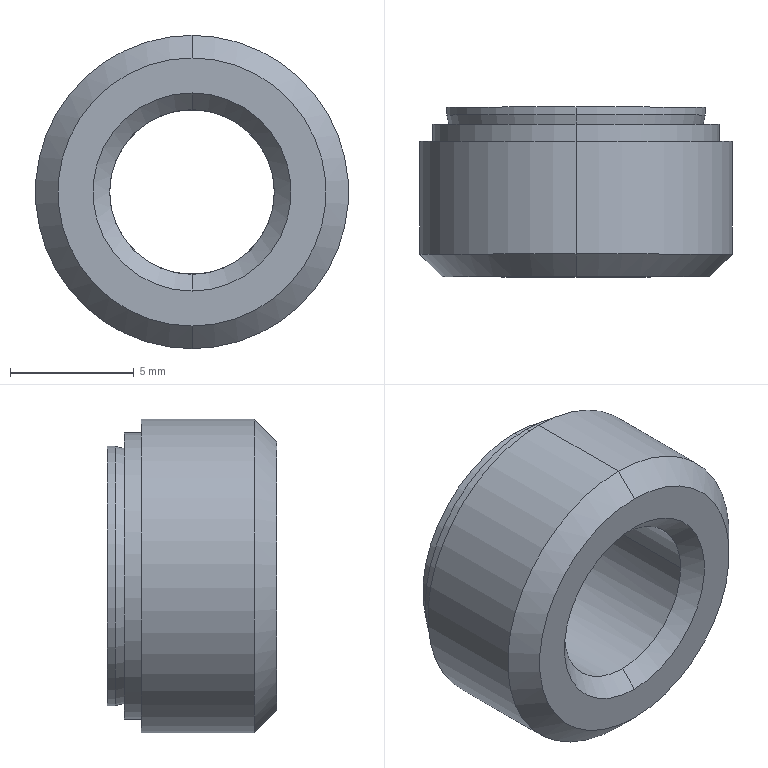Part | NX | features solid 2 | 1 solid | 20 faces | box 12.65 x 6.85 x 12.65 mm | volume 555.144 mm3 | cone 8 | cylinder 8 | plane 4 | commonest cylinder face diameters 6.647 x2 10.47 x2 11.56 x2 12.65 x2
STEP:
#1=CARTESIAN_POINT('',(107.,-8.66,-1026.113));
#2=VERTEX_POINT('',#1);
#3=CARTESIAN_POINT('',(107.,-8.66,-1015.287));
#4=VERTEX_POINT('',#3);
#5=CARTESIAN_POINT('',(107.,-8.66,-1020.7));
#6=DIRECTION('',(0.,1.,0.));
#7=DIRECTION('',(0.,0.,-1.));
#8=AXIS2_PLACEMENT_3D('',#5,#6,#7);
#9=CIRCLE('',#8,5.413);
#10=EDGE_CURVE('',#2,#4,#9,.T.);
#11=ORIENTED_EDGE('',*,*,#10,.T.);
#12=CARTESIAN_POINT('',(107.,-7.748,-1014.375));
#13=VERTEX_POINT('',#12);
#14=CARTESIAN_POINT('',(107.,-7.748,-1014.375));
#15=DIRECTION('',(0.,-0.7071,-0.7071));
#16=VECTOR('',#15,1000.);
#17=LINE('',#14,#16);
#18=EDGE_CURVE('',#4,#13,#17,.F.);
#19=ORIENTED_EDGE('',*,*,#18,.T.);
#20=CARTESIAN_POINT('',(107.,-7.748,-1027.025));
#21=VERTEX_POINT('',#20);
#22=CARTESIAN_POINT('',(107.,-7.748,-1020.7));
#23=DIRECTION('',(0.,1.,0.));
#24=DIRECTION('',(0.,0.,-1.));
#25=AXIS2_PLACEMENT_3D('',#22,#23,#24);
#26=CIRCLE('',#25,6.325);
#27=EDGE_CURVE('',#21,#13,#26,.T.);
#28=ORIENTED_EDGE('',*,*,#27,.F.);
#29=CARTESIAN_POINT('',(107.,-7.748,-1027.025));
#30=DIRECTION('',(0.,-0.7071,0.7071));
#31=VECTOR('',#30,1000.);
#32=LINE('',#29,#31);
#33=EDGE_CURVE('',#21,#2,#32,.T.);
#34=ORIENTED_EDGE('',*,*,#33,.T.);
#35=EDGE_LOOP('',(#11,#19,#28,#34));
#36=FACE_BOUND('',#35,.T.);
#37=CARTESIAN_POINT('',(107.,-8.204,-1020.7));
#38=DIRECTION('',(0.,1.,0.));
#39=DIRECTION('',(0.,0.,-1.));
#40=AXIS2_PLACEMENT_3D('',#37,#38,#39);
#41=CONICAL_SURFACE('',#40,5.869,0.7854);
#42=ADVANCED_FACE('',(#36),#41,.T.);
#43=ORIENTED_EDGE('',*,*,#33,.F.);
#44=CARTESIAN_POINT('',(107.,-7.748,-1020.7));
#45=DIRECTION('',(0.,1.,0.));
#46=DIRECTION('',(0.,0.,1.));
#47=AXIS2_PLACEMENT_3D('',#44,#45,#46);
#48=CIRCLE('',#47,6.325);
#49=EDGE_CURVE('',#13,#21,#48,.T.);
#50=ORIENTED_EDGE('',*,*,#49,.F.);
#51=ORIENTED_EDGE('',*,*,#18,.F.);
#52=CARTESIAN_POINT('',(107.,-8.66,-1020.7));
#53=DIRECTION('',(0.,1.,0.));
#54=DIRECTION('',(0.,0.,1.));
#55=AXIS2_PLACEMENT_3D('',#52,#53,#54);
#56=CIRCLE('',#55,5.413);
#57=EDGE_CURVE('',#4,#2,#56,.T.);
#58=ORIENTED_EDGE('',*,*,#57,.T.);
#59=EDGE_LOOP('',(#43,#50,#51,#58));
#60=FACE_BOUND('',#59,.T.);
#61=CARTESIAN_POINT('',(107.,-8.204,-1020.7));
#62=DIRECTION('',(0.,1.,0.));
#63=DIRECTION('',(0.,0.,-1.));
#64=AXIS2_PLACEMENT_3D('',#61,#62,#63);
#65=CONICAL_SURFACE('',#64,5.869,0.7854);
#66=ADVANCED_FACE('',(#60),#65,.T.);
#67=ORIENTED_EDGE('',*,*,#10,.F.);
#68=ORIENTED_EDGE('',*,*,#57,.F.);
#69=EDGE_LOOP('',(#67,#68));
#70=FACE_BOUND('',#69,.T.);
#71=CARTESIAN_POINT('',(107.,-8.66,-1024.7));
#72=VERTEX_POINT('',#71);
#73=CARTESIAN_POINT('',(107.,-8.66,-1016.7));
#74=VERTEX_POINT('',#73);
#75=CARTESIAN_POINT('',(107.,-8.66,-1020.7));
#76=DIRECTION('',(0.,-1.,0.));
#77=DIRECTION('',(0.,0.,-1.));
#78=AXIS2_PLACEMENT_3D('',#75,#76,#77);
#79=CIRCLE('',#78,4.);
#80=EDGE_CURVE('',#72,#74,#79,.T.);
#81=ORIENTED_EDGE('',*,*,#80,.F.);
#82=CARTESIAN_POINT('',(107.,-8.66,-1020.7));
#83=DIRECTION('',(0.,-1.,0.));
#84=DIRECTION('',(0.,0.,1.));
#85=AXIS2_PLACEMENT_3D('',#82,#83,#84);
#86=CIRCLE('',#85,4.);
#87=EDGE_CURVE('',#74,#72,#86,.T.);
#88=ORIENTED_EDGE('',*,*,#87,.F.);
#89=EDGE_LOOP('',(#81,#88));
#90=FACE_BOUND('',#89,.T.);
#91=CARTESIAN_POINT('',(107.,-8.66,-1017.993));
#92=DIRECTION('',(0.,-1.,0.));
#93=DIRECTION('',(-1.,0.,0.));
#94=AXIS2_PLACEMENT_3D('',#91,#92,#93);
#95=PLANE('',#94);
#96=ADVANCED_FACE('',(#70,#90),#95,.T.);
#97=CARTESIAN_POINT('',(107.,-7.984,-1017.377));
#98=VERTEX_POINT('',#97);
#99=CARTESIAN_POINT('',(107.,-8.66,-1016.7));
#100=DIRECTION('',(0.,0.7071,-0.7071));
#101=VECTOR('',#100,1000.);
#102=LINE('',#99,#101);
#103=EDGE_CURVE('',#74,#98,#102,.T.);
#104=ORIENTED_EDGE('',*,*,#103,.F.);
#105=ORIENTED_EDGE('',*,*,#87,.T.);
#106=CARTESIAN_POINT('',(107.,-7.984,-1024.023));
#107=VERTEX_POINT('',#106);
#108=CARTESIAN_POINT('',(107.,-8.66,-1024.7));
#109=DIRECTION('',(0.,0.7071,0.7071));
#110=VECTOR('',#109,1000.);
#111=LINE('',#108,#110);
#112=EDGE_CURVE('',#107,#72,#111,.F.);
#113=ORIENTED_EDGE('',*,*,#112,.F.);
#114=CARTESIAN_POINT('',(103.677,-7.984,-1020.7));
#115=VERTEX_POINT('',#114);
#116=CARTESIAN_POINT('',(107.,-7.984,-1020.7));
#117=DIRECTION('',(0.,-1.,0.));
#118=DIRECTION('',(-1.,0.,0.));
#119=AXIS2_PLACEMENT_3D('',#116,#117,#118);
#120=CIRCLE('',#119,3.323);
#121=EDGE_CURVE('',#115,#107,#120,.T.);
#122=ORIENTED_EDGE('',*,*,#121,.F.);
#123=CARTESIAN_POINT('',(107.,-7.984,-1020.7));
#124=DIRECTION('',(0.,-1.,0.));
#125=DIRECTION('',(0.,0.,1.));
#126=AXIS2_PLACEMENT_3D('',#123,#124,#125);
#127=CIRCLE('',#126,3.323);
#128=EDGE_CURVE('',#98,#115,#127,.T.);
#129=ORIENTED_EDGE('',*,*,#128,.F.);
#130=EDGE_LOOP('',(#104,#105,#113,#122,#129));
#131=FACE_BOUND('',#130,.T.);
#132=CARTESIAN_POINT('',(107.,-8.322,-1020.7));
#133=DIRECTION('',(0.,-1.,0.));
#134=DIRECTION('',(0.,0.,1.));
#135=AXIS2_PLACEMENT_3D('',#132,#133,#134);
#136=CONICAL_SURFACE('',#135,3.662,0.7854);
#137=ADVANCED_FACE('',(#131),#136,.F.);
#138=CARTESIAN_POINT('',(110.323,-7.984,-1020.7));
#139=VERTEX_POINT('',#138);
#140=CARTESIAN_POINT('',(107.,-7.984,-1020.7));
#141=DIRECTION('',(0.,-1.,0.));
#142=DIRECTION('',(1.,0.,0.));
#143=AXIS2_PLACEMENT_3D('',#140,#141,#142);
#144=CIRCLE('',#143,3.323);
#145=EDGE_CURVE('',#139,#98,#144,.T.);
#146=ORIENTED_EDGE('',*,*,#145,.T.);
#147=ORIENTED_EDGE('',*,*,#128,.T.);
#148=CARTESIAN_POINT('',(103.676,-2.487,-1020.7));
#149=VERTEX_POINT('',#148);
#150=CARTESIAN_POINT('',(103.676,-2.487,-1020.7));
#151=DIRECTION('',(0.,-1.,0.));
#152=VECTOR('',#151,1000.);
#153=LINE('',#150,#152);
#154=EDGE_CURVE('',#149,#115,#153,.T.);
#155=ORIENTED_EDGE('',*,*,#154,.F.);
#156=CARTESIAN_POINT('',(110.324,-2.487,-1020.7));
#157=VERTEX_POINT('',#156);
#158=CARTESIAN_POINT('',(107.,-2.487,-1020.7));
#159=DIRECTION('',(0.,1.,0.));
#160=DIRECTION('',(-1.,0.,0.));
#161=AXIS2_PLACEMENT_3D('',#158,#159,#160);
#162=CIRCLE('',#161,3.324);
#163=EDGE_CURVE('',#149,#157,#162,.T.);
#164=ORIENTED_EDGE('',*,*,#163,.T.);
#165=CARTESIAN_POINT('',(110.324,-2.487,-1020.7));
#166=DIRECTION('',(0.,-1.,0.));
#167=VECTOR('',#166,1000.);
#168=LINE('',#165,#167);
#169=EDGE_CURVE('',#139,#157,#168,.F.);
#170=ORIENTED_EDGE('',*,*,#169,.F.);
#171=EDGE_LOOP('',(#146,#147,#155,#164,#170));
#172=FACE_BOUND('',#171,.T.);
#173=CARTESIAN_POINT('',(107.,-7.984,-1020.7));
#174=DIRECTION('',(0.,1.,0.));
#175=DIRECTION('',(1.,0.,0.));
#176=AXIS2_PLACEMENT_3D('',#173,#174,#175);
#177=CYLINDRICAL_SURFACE('',#176,3.324);
#178=ADVANCED_FACE('',(#172),#177,.F.);
#179=ORIENTED_EDGE('',*,*,#169,.T.);
#180=CARTESIAN_POINT('',(107.,-2.487,-1020.7));
#181=DIRECTION('',(0.,1.,0.));
#182=DIRECTION('',(1.,0.,0.));
#183=AXIS2_PLACEMENT_3D('',#180,#181,#182);
#184=CIRCLE('',#183,3.324);
#185=EDGE_CURVE('',#157,#149,#184,.T.);
#186=ORIENTED_EDGE('',*,*,#185,.T.);
#187=ORIENTED_EDGE('',*,*,#154,.T.);
#188=ORIENTED_EDGE('',*,*,#121,.T.);
#189=CARTESIAN_POINT('',(107.,-7.984,-1020.7));
#190=DIRECTION('',(0.,-1.,0.));
#191=DIRECTION('',(0.,0.,-1.));
#192=AXIS2_PLACEMENT_3D('',#189,#190,#191);
#193=CIRCLE('',#192,3.323);
#194=EDGE_CURVE('',#107,#139,#193,.T.);
#195=ORIENTED_EDGE('',*,*,#194,.T.);
#196=EDGE_LOOP('',(#179,#186,#187,#188,#195));
#197=FACE_BOUND('',#196,.T.);
#198=CARTESIAN_POINT('',(107.,-7.984,-1020.7));
#199=DIRECTION('',(0.,1.,0.));
#200=DIRECTION('',(1.,0.,0.));
#201=AXIS2_PLACEMENT_3D('',#198,#199,#200);
#202=CYLINDRICAL_SURFACE('',#201,3.324);
#203=ADVANCED_FACE('',(#197),#202,.F.);
#204=ORIENTED_EDGE('',*,*,#145,.F.);
#205=ORIENTED_EDGE('',*,*,#194,.F.);
#206=ORIENTED_EDGE('',*,*,#112,.T.);
#207=ORIENTED_EDGE('',*,*,#80,.T.);
#208=ORIENTED_EDGE('',*,*,#103,.T.);
#209=EDGE_LOOP('',(#204,#205,#206,#207,#208));
#210=FACE_BOUND('',#209,.T.);
#211=CARTESIAN_POINT('',(107.,-8.322,-1020.7));
#212=DIRECTION('',(0.,-1.,0.));
#213=DIRECTION('',(0.,0.,1.));
#214=AXIS2_PLACEMENT_3D('',#211,#212,#213);
#215=CONICAL_SURFACE('',#214,3.662,0.7854);
#216=ADVANCED_FACE('',(#210),#215,.F.);
#217=CARTESIAN_POINT('',(111.,-1.81,-1020.7));
#218=VERTEX_POINT('',#217);
#219=CARTESIAN_POINT('',(111.,-1.81,-1020.7));
#220=DIRECTION('',(-0.7071,-0.7071,0.));
#221=VECTOR('',#220,1000.);
#222=LINE('',#219,#221);
#223=EDGE_CURVE('',#157,#218,#222,.F.);
#224=ORIENTED_EDGE('',*,*,#223,.T.);
#225=CARTESIAN_POINT('',(103.,-1.81,-1020.7));
#226=VERTEX_POINT('',#225);
#227=CARTESIAN_POINT('',(107.,-1.81,-1020.7));
#228=DIRECTION('',(0.,1.,0.));
#229=DIRECTION('',(1.,0.,0.));
#230=AXIS2_PLACEMENT_3D('',#227,#228,#229);
#231=CIRCLE('',#230,4.);
#232=EDGE_CURVE('',#218,#226,#231,.T.);
#233=ORIENTED_EDGE('',*,*,#232,.T.);
#234=CARTESIAN_POINT('',(103.,-1.81,-1020.7));
#235=DIRECTION('',(0.7071,-0.7071,0.));
#236=VECTOR('',#235,1000.);
#237=LINE('',#234,#236);
#238=EDGE_CURVE('',#226,#149,#237,.T.);
#239=ORIENTED_EDGE('',*,*,#238,.T.);
#240=ORIENTED_EDGE('',*,*,#185,.F.);
#241=EDGE_LOOP('',(#224,#233,#239,#240));
#242=FACE_BOUND('',#241,.T.);
#243=CARTESIAN_POINT('',(107.,-2.148,-1020.7));
#244=DIRECTION('',(0.,1.,0.));
#245=DIRECTION('',(1.,0.,0.));
#246=AXIS2_PLACEMENT_3D('',#243,#244,#245);
#247=CONICAL_SURFACE('',#246,3.662,0.7854);
#248=ADVANCED_FACE('',(#242),#247,.F.);
#249=ORIENTED_EDGE('',*,*,#163,.F.);
#250=ORIENTED_EDGE('',*,*,#238,.F.);
#251=CARTESIAN_POINT('',(107.,-1.81,-1020.7));
#252=DIRECTION('',(0.,1.,0.));
#253=DIRECTION('',(-1.,0.,0.));
#254=AXIS2_PLACEMENT_3D('',#251,#252,#253);
#255=CIRCLE('',#254,4.);
#256=EDGE_CURVE('',#226,#218,#255,.T.);
#257=ORIENTED_EDGE('',*,*,#256,.T.);
#258=ORIENTED_EDGE('',*,*,#223,.F.);
#259=EDGE_LOOP('',(#249,#250,#257,#258));
#260=FACE_BOUND('',#259,.T.);
#261=CARTESIAN_POINT('',(107.,-2.148,-1020.7));
#262=DIRECTION('',(0.,1.,0.));
#263=DIRECTION('',(1.,0.,0.));
#264=AXIS2_PLACEMENT_3D('',#261,#262,#263);
#265=CONICAL_SURFACE('',#264,3.662,0.7854);
#266=ADVANCED_FACE('',(#260),#265,.F.);
#267=CARTESIAN_POINT('',(107.,-1.81,-1015.465));
#268=VERTEX_POINT('',#267);
#269=CARTESIAN_POINT('',(107.,-1.81,-1025.935));
#270=VERTEX_POINT('',#269);
#271=CARTESIAN_POINT('',(107.,-1.81,-1020.7));
#272=DIRECTION('',(0.,-1.,0.));
#273=DIRECTION('',(0.,0.,1.));
#274=AXIS2_PLACEMENT_3D('',#271,#272,#273);
#275=CIRCLE('',#274,5.235);
#276=EDGE_CURVE('',#268,#270,#275,.T.);
#277=ORIENTED_EDGE('',*,*,#276,.F.);
#278=CARTESIAN_POINT('',(107.,-1.81,-1020.7));
#279=DIRECTION('',(0.,-1.,0.));
#280=DIRECTION('',(0.,0.,-1.));
#281=AXIS2_PLACEMENT_3D('',#278,#279,#280);
#282=CIRCLE('',#281,5.235);
#283=EDGE_CURVE('',#270,#268,#282,.T.);
#284=ORIENTED_EDGE('',*,*,#283,.F.);
#285=EDGE_LOOP('',(#277,#284));
#286=FACE_BOUND('',#285,.T.);
#287=ORIENTED_EDGE('',*,*,#232,.F.);
#288=ORIENTED_EDGE('',*,*,#256,.F.);
#289=EDGE_LOOP('',(#287,#288));
#290=FACE_BOUND('',#289,.T.);
#291=CARTESIAN_POINT('',(107.,-1.81,-1018.082));
#292=DIRECTION('',(0.,1.,0.));
#293=DIRECTION('',(0.,0.,-1.));
#294=AXIS2_PLACEMENT_3D('',#291,#292,#293);
#295=PLANE('',#294);
#296=ADVANCED_FACE('',(#286,#290),#295,.T.);
#297=CARTESIAN_POINT('',(107.,-2.128,-1015.465));
#298=VERTEX_POINT('',#297);
#299=CARTESIAN_POINT('',(107.,-2.128,-1015.465));
#300=DIRECTION('',(0.,1.,0.));
#301=VECTOR('',#300,1000.);
#302=LINE('',#299,#301);
#303=EDGE_CURVE('',#268,#298,#302,.F.);
#304=ORIENTED_EDGE('',*,*,#303,.T.);
#305=CARTESIAN_POINT('',(107.,-2.128,-1025.935));
#306=VERTEX_POINT('',#305);
#307=CARTESIAN_POINT('',(107.,-2.128,-1020.7));
#308=DIRECTION('',(0.,1.,0.));
#309=DIRECTION('',(0.,0.,1.));
#310=AXIS2_PLACEMENT_3D('',#307,#308,#309);
#311=CIRCLE('',#310,5.235);
#312=EDGE_CURVE('',#298,#306,#311,.T.);
#313=ORIENTED_EDGE('',*,*,#312,.T.);
#314=CARTESIAN_POINT('',(107.,-2.128,-1025.935));
#315=DIRECTION('',(0.,1.,0.));
#316=VECTOR('',#315,1000.);
#317=LINE('',#314,#316);
#318=EDGE_CURVE('',#306,#270,#317,.T.);
#319=ORIENTED_EDGE('',*,*,#318,.T.);
#320=ORIENTED_EDGE('',*,*,#283,.T.);
#321=EDGE_LOOP('',(#304,#313,#319,#320));
#322=FACE_BOUND('',#321,.T.);
#323=CARTESIAN_POINT('',(107.,-1.969,-1020.7));
#324=DIRECTION('',(0.,-1.,0.));
#325=DIRECTION('',(0.,0.,1.));
#326=AXIS2_PLACEMENT_3D('',#323,#324,#325);
#327=CYLINDRICAL_SURFACE('',#326,5.235);
#328=ADVANCED_FACE('',(#322),#327,.T.);
#329=ORIENTED_EDGE('',*,*,#276,.T.);
#330=ORIENTED_EDGE('',*,*,#318,.F.);
#331=CARTESIAN_POINT('',(107.,-2.128,-1020.7));
#332=DIRECTION('',(0.,1.,0.));
#333=DIRECTION('',(0.,0.,-1.));
#334=AXIS2_PLACEMENT_3D('',#331,#332,#333);
#335=CIRCLE('',#334,5.235);
#336=EDGE_CURVE('',#306,#298,#335,.T.);
#337=ORIENTED_EDGE('',*,*,#336,.T.);
#338=ORIENTED_EDGE('',*,*,#303,.F.);
#339=EDGE_LOOP('',(#329,#330,#337,#338));
#340=FACE_BOUND('',#339,.T.);
#341=CARTESIAN_POINT('',(107.,-1.969,-1020.7));
#342=DIRECTION('',(0.,-1.,0.));
#343=DIRECTION('',(0.,0.,1.));
#344=AXIS2_PLACEMENT_3D('',#341,#342,#343);
#345=CYLINDRICAL_SURFACE('',#344,5.235);
#346=ADVANCED_FACE('',(#340),#345,.T.);
#347=CARTESIAN_POINT('',(107.,-2.5,-1025.848));
#348=VERTEX_POINT('',#347);
#349=CARTESIAN_POINT('',(107.,-2.5,-1015.552));
#350=VERTEX_POINT('',#349);
#351=CARTESIAN_POINT('',(107.,-2.5,-1020.7));
#352=DIRECTION('',(0.,1.,0.));
#353=DIRECTION('',(0.,0.,-1.));
#354=AXIS2_PLACEMENT_3D('',#351,#352,#353);
#355=CIRCLE('',#354,5.148);
#356=EDGE_CURVE('',#348,#350,#355,.T.);
#357=ORIENTED_EDGE('',*,*,#356,.T.);
#358=CARTESIAN_POINT('',(107.,-2.128,-1015.465));
#359=DIRECTION('',(0.,-0.9735,-0.2286));
#360=VECTOR('',#359,1000.);
#361=LINE('',#358,#360);
#362=EDGE_CURVE('',#350,#298,#361,.F.);
#363=ORIENTED_EDGE('',*,*,#362,.T.);
#364=ORIENTED_EDGE('',*,*,#336,.F.);
#365=CARTESIAN_POINT('',(107.,-2.128,-1025.935));
#366=DIRECTION('',(0.,-0.9735,0.2286));
#367=VECTOR('',#366,1000.);
#368=LINE('',#365,#367);
#369=EDGE_CURVE('',#306,#348,#368,.T.);
#370=ORIENTED_EDGE('',*,*,#369,.T.);
#371=EDGE_LOOP('',(#357,#363,#364,#370));
#372=FACE_BOUND('',#371,.T.);
#373=CARTESIAN_POINT('',(107.,-2.314,-1020.7));
#374=DIRECTION('',(0.,1.,0.));
#375=DIRECTION('',(0.,0.,-1.));
#376=AXIS2_PLACEMENT_3D('',#373,#374,#375);
#377=CONICAL_SURFACE('',#376,5.191,0.2307);
#378=ADVANCED_FACE('',(#372),#377,.T.);
#379=ORIENTED_EDGE('',*,*,#369,.F.);
#380=ORIENTED_EDGE('',*,*,#312,.F.);
#381=ORIENTED_EDGE('',*,*,#362,.F.);
#382=CARTESIAN_POINT('',(107.,-2.5,-1020.7));
#383=DIRECTION('',(0.,1.,0.));
#384=DIRECTION('',(0.,0.,1.));
#385=AXIS2_PLACEMENT_3D('',#382,#383,#384);
#386=CIRCLE('',#385,5.148);
#387=EDGE_CURVE('',#350,#348,#386,.T.);
#388=ORIENTED_EDGE('',*,*,#387,.T.);
#389=EDGE_LOOP('',(#379,#380,#381,#388));
#390=FACE_BOUND('',#389,.T.);
#391=CARTESIAN_POINT('',(107.,-2.314,-1020.7));
#392=DIRECTION('',(0.,1.,0.));
#393=DIRECTION('',(0.,0.,-1.));
#394=AXIS2_PLACEMENT_3D('',#391,#392,#393);
#395=CONICAL_SURFACE('',#394,5.191,0.2307);
#396=ADVANCED_FACE('',(#390),#395,.T.);
#397=CARTESIAN_POINT('',(107.,-2.5,-1026.48));
#398=VERTEX_POINT('',#397);
#399=CARTESIAN_POINT('',(107.,-2.5,-1014.92));
#400=VERTEX_POINT('',#399);
#401=CARTESIAN_POINT('',(107.,-2.5,-1020.7));
#402=DIRECTION('',(0.,-1.,0.));
#403=DIRECTION('',(0.,0.,-1.));
#404=AXIS2_PLACEMENT_3D('',#401,#402,#403);
#405=CIRCLE('',#404,5.78);
#406=EDGE_CURVE('',#398,#400,#405,.T.);
#407=ORIENTED_EDGE('',*,*,#406,.F.);
#408=CARTESIAN_POINT('',(107.,-2.5,-1020.7));
#409=DIRECTION('',(0.,-1.,0.));
#410=DIRECTION('',(0.,0.,1.));
#411=AXIS2_PLACEMENT_3D('',#408,#409,#410);
#412=CIRCLE('',#411,5.78);
#413=EDGE_CURVE('',#400,#398,#412,.T.);
#414=ORIENTED_EDGE('',*,*,#413,.F.);
#415=EDGE_LOOP('',(#407,#414));
#416=FACE_BOUND('',#415,.T.);
#417=ORIENTED_EDGE('',*,*,#387,.F.);
#418=ORIENTED_EDGE('',*,*,#356,.F.);
#419=EDGE_LOOP('',(#417,#418));
#420=FACE_BOUND('',#419,.T.);
#421=CARTESIAN_POINT('',(107.,-2.5,-1020.7));
#422=DIRECTION('',(0.,1.,0.));
#423=DIRECTION('',(0.,0.,-1.));
#424=AXIS2_PLACEMENT_3D('',#421,#422,#423);
#425=PLANE('',#424);
#426=ADVANCED_FACE('',(#416,#420),#425,.T.);
#427=CARTESIAN_POINT('',(107.,-3.19,-1026.48));
#428=VERTEX_POINT('',#427);
#429=CARTESIAN_POINT('',(107.,-3.19,-1014.92));
#430=VERTEX_POINT('',#429);
#431=CARTESIAN_POINT('',(107.,-3.19,-1020.7));
#432=DIRECTION('',(0.,1.,0.));
#433=DIRECTION('',(0.,0.,-1.));
#434=AXIS2_PLACEMENT_3D('',#431,#432,#433);
#435=CIRCLE('',#434,5.78);
#436=EDGE_CURVE('',#428,#430,#435,.T.);
#437=ORIENTED_EDGE('',*,*,#436,.T.);
#438=CARTESIAN_POINT('',(107.,-2.5,-1014.92));
#439=DIRECTION('',(0.,-1.,0.));
#440=VECTOR('',#439,1000.);
#441=LINE('',#438,#440);
#442=EDGE_CURVE('',#400,#430,#441,.T.);
#443=ORIENTED_EDGE('',*,*,#442,.F.);
#444=ORIENTED_EDGE('',*,*,#413,.T.);
#445=CARTESIAN_POINT('',(107.,-2.5,-1026.48));
#446=DIRECTION('',(0.,-1.,0.));
#447=VECTOR('',#446,1000.);
#448=LINE('',#445,#447);
#449=EDGE_CURVE('',#428,#398,#448,.F.);
#450=ORIENTED_EDGE('',*,*,#449,.F.);
#451=EDGE_LOOP('',(#437,#443,#444,#450));
#452=FACE_BOUND('',#451,.T.);
#453=CARTESIAN_POINT('',(107.,-2.845,-1020.7));
#454=DIRECTION('',(0.,1.,0.));
#455=DIRECTION('',(0.,0.,-1.));
#456=AXIS2_PLACEMENT_3D('',#453,#454,#455);
#457=CYLINDRICAL_SURFACE('',#456,5.78);
#458=ADVANCED_FACE('',(#452),#457,.T.);
#459=ORIENTED_EDGE('',*,*,#449,.T.);
#460=ORIENTED_EDGE('',*,*,#406,.T.);
#461=ORIENTED_EDGE('',*,*,#442,.T.);
#462=CARTESIAN_POINT('',(107.,-3.19,-1020.7));
#463=DIRECTION('',(0.,1.,0.));
#464=DIRECTION('',(0.,0.,1.));
#465=AXIS2_PLACEMENT_3D('',#462,#463,#464);
#466=CIRCLE('',#465,5.78);
#467=EDGE_CURVE('',#430,#428,#466,.T.);
#468=ORIENTED_EDGE('',*,*,#467,.T.);
#469=EDGE_LOOP('',(#459,#460,#461,#468));
#470=FACE_BOUND('',#469,.T.);
#471=CARTESIAN_POINT('',(107.,-2.845,-1020.7));
#472=DIRECTION('',(0.,1.,0.));
#473=DIRECTION('',(0.,0.,-1.));
#474=AXIS2_PLACEMENT_3D('',#471,#472,#473);
#475=CYLINDRICAL_SURFACE('',#474,5.78);
#476=ADVANCED_FACE('',(#470),#475,.T.);
#477=CARTESIAN_POINT('',(107.,-3.19,-1014.375));
#478=VERTEX_POINT('',#477);
#479=CARTESIAN_POINT('',(107.,-3.19,-1027.025));
#480=VERTEX_POINT('',#479);
#481=CARTESIAN_POINT('',(107.,-3.19,-1020.7));
#482=DIRECTION('',(0.,-1.,0.));
#483=DIRECTION('',(0.,0.,1.));
#484=AXIS2_PLACEMENT_3D('',#481,#482,#483);
#485=CIRCLE('',#484,6.325);
#486=EDGE_CURVE('',#478,#480,#485,.T.);
#487=ORIENTED_EDGE('',*,*,#486,.F.);
#488=CARTESIAN_POINT('',(107.,-3.19,-1020.7));
#489=DIRECTION('',(0.,-1.,0.));
#490=DIRECTION('',(0.,0.,-1.));
#491=AXIS2_PLACEMENT_3D('',#488,#489,#490);
#492=CIRCLE('',#491,6.325);
#493=EDGE_CURVE('',#480,#478,#492,.T.);
#494=ORIENTED_EDGE('',*,*,#493,.F.);
#495=EDGE_LOOP('',(#487,#494));
#496=FACE_BOUND('',#495,.T.);
#497=ORIENTED_EDGE('',*,*,#467,.F.);
#498=ORIENTED_EDGE('',*,*,#436,.F.);
#499=EDGE_LOOP('',(#497,#498));
#500=FACE_BOUND('',#499,.T.);
#501=CARTESIAN_POINT('',(107.,-3.19,-1017.538));
#502=DIRECTION('',(0.,1.,0.));
#503=DIRECTION('',(0.,0.,-1.));
#504=AXIS2_PLACEMENT_3D('',#501,#502,#503);
#505=PLANE('',#504);
#506=ADVANCED_FACE('',(#496,#500),#505,.T.);
#507=CARTESIAN_POINT('',(107.,-7.748,-1014.375));
#508=DIRECTION('',(0.,1.,0.));
#509=VECTOR('',#508,1000.);
#510=LINE('',#507,#509);
#511=EDGE_CURVE('',#13,#478,#510,.T.);
#512=ORIENTED_EDGE('',*,*,#511,.F.);
#513=ORIENTED_EDGE('',*,*,#49,.T.);
#514=CARTESIAN_POINT('',(107.,-7.748,-1027.025));
#515=DIRECTION('',(0.,1.,0.));
#516=VECTOR('',#515,1000.);
#517=LINE('',#514,#516);
#518=EDGE_CURVE('',#480,#21,#517,.F.);
#519=ORIENTED_EDGE('',*,*,#518,.F.);
#520=ORIENTED_EDGE('',*,*,#493,.T.);
#521=EDGE_LOOP('',(#512,#513,#519,#520));
#522=FACE_BOUND('',#521,.T.);
#523=CARTESIAN_POINT('',(107.,-5.469,-1020.7));
#524=DIRECTION('',(0.,-1.,0.));
#525=DIRECTION('',(0.,0.,1.));
#526=AXIS2_PLACEMENT_3D('',#523,#524,#525);
#527=CYLINDRICAL_SURFACE('',#526,6.325);
#528=ADVANCED_FACE('',(#522),#527,.T.);
#529=ORIENTED_EDGE('',*,*,#486,.T.);
#530=ORIENTED_EDGE('',*,*,#518,.T.);
#531=ORIENTED_EDGE('',*,*,#27,.T.);
#532=ORIENTED_EDGE('',*,*,#511,.T.);
#533=EDGE_LOOP('',(#529,#530,#531,#532));
#534=FACE_BOUND('',#533,.T.);
#535=CARTESIAN_POINT('',(107.,-5.469,-1020.7));
#536=DIRECTION('',(0.,-1.,0.));
#537=DIRECTION('',(0.,0.,1.));
#538=AXIS2_PLACEMENT_3D('',#535,#536,#537);
#539=CYLINDRICAL_SURFACE('',#538,6.325);
#540=ADVANCED_FACE('',(#534),#539,.T.);
#541=CLOSED_SHELL('',(#42,#66,#96,#137,#178,#203,#216,#248,#266,#296,#328,#346,#378,#396,#426,#458,#476,#506,#528,#540));
#542=MANIFOLD_SOLID_BREP('',#541);
#543=(LENGTH_UNIT()NAMED_UNIT(*)SI_UNIT(.MILLI.,.METRE.));
#544=UNCERTAINTY_MEASURE_WITH_UNIT(LENGTH_MEASURE(0.00001),#543,'','');
#545=(NAMED_UNIT(*)PLANE_ANGLE_UNIT()SI_UNIT($,.RADIAN.));
#546=(NAMED_UNIT(*)SI_UNIT($,.STERADIAN.)SOLID_ANGLE_UNIT());
#547=(GEOMETRIC_REPRESENTATION_CONTEXT(3)GLOBAL_UNCERTAINTY_ASSIGNED_CONTEXT((#544))GLOBAL_UNIT_ASSIGNED_CONTEXT((#543,#545,#546))REPRESENTATION_CONTEXT('',''));
#548=ADVANCED_BREP_SHAPE_REPRESENTATION('',(#542),#547);